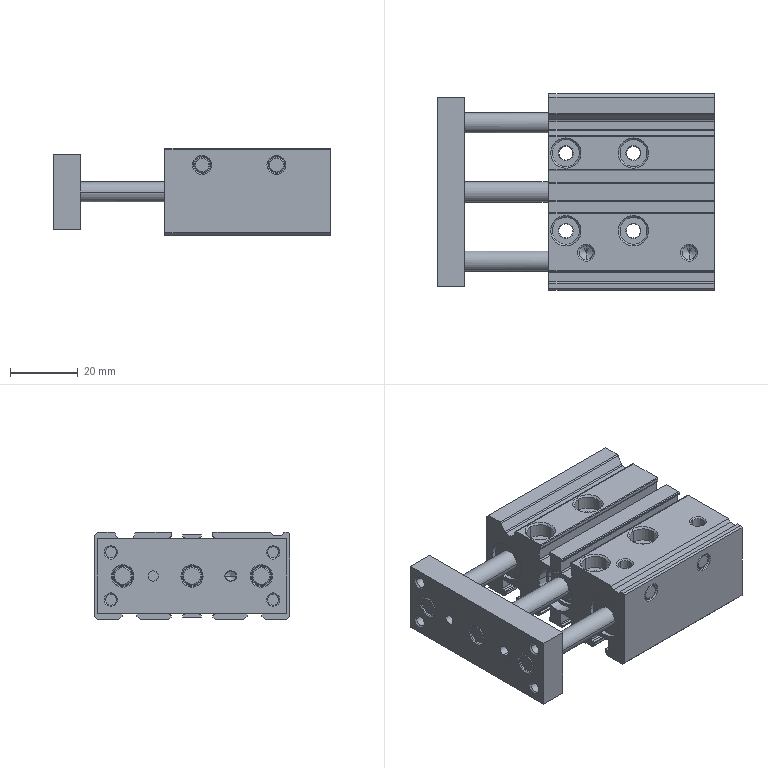Part | SolidWorks | 2 solids | 371 faces | box 82 x 58 x 26 mm | volume 65223 mm3 | cylinder 161 | plane 122 | cone 86 | spline 2 | commonest cylinder face diameters 3 x21 0.8 x20 6 x18 3.242 x16 0.4 x12 4.134 x12